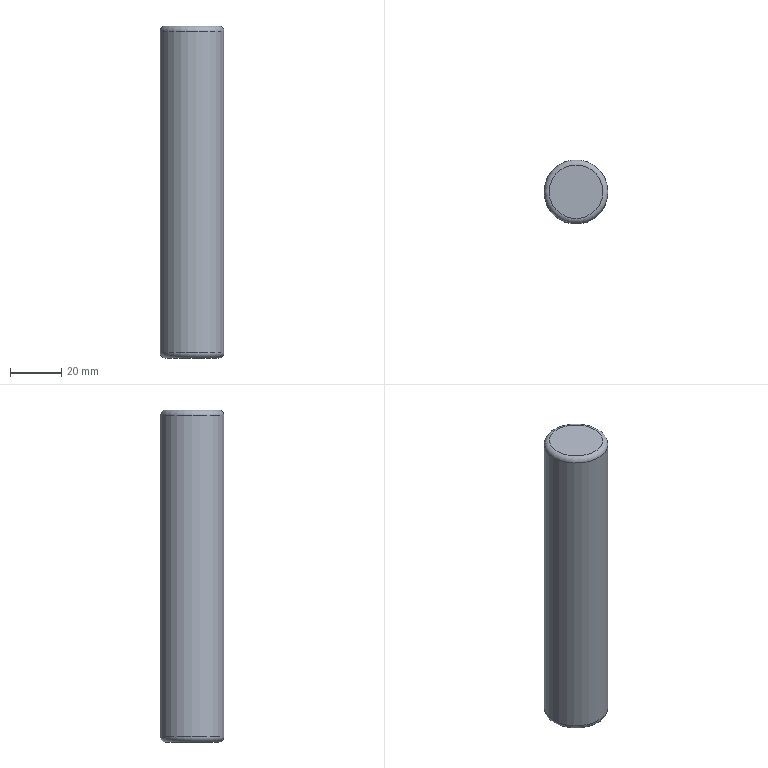Part | NX | features BLEND 1, CYLINDER 1, DATUM_CSYS 1 | 1 solid | 5 faces | box 25 x 25 x 130 mm | volume 63684 mm3 | plane 2 | torus 2 | cylinder 1 | commonest cylinder face diameters 25 x1
STEP:
#1=CARTESIAN_POINT('',(10.5,0.,130.));
#2=VERTEX_POINT('',#1);
#3=CARTESIAN_POINT('',(0.,0.,130.));
#4=DIRECTION('',(0.,0.,1.));
#5=DIRECTION('',(1.,0.,0.));
#6=AXIS2_PLACEMENT_3D('',#3,#4,#5);
#7=CIRCLE('',#6,10.5);
#8=EDGE_CURVE('',#2,#2,#7,.T.);
#9=ORIENTED_EDGE('',*,*,#8,.T.);
#10=EDGE_LOOP('',(#9));
#11=FACE_BOUND('',#10,.T.);
#12=CARTESIAN_POINT('',(0.,0.,130.));
#13=DIRECTION('',(0.,0.,1.));
#14=DIRECTION('',(1.,0.,0.));
#15=AXIS2_PLACEMENT_3D('',#12,#13,#14);
#16=PLANE('',#15);
#17=ADVANCED_FACE('',(#11),#16,.T.);
#18=CARTESIAN_POINT('',(-10.5,0.,0.));
#19=VERTEX_POINT('',#18);
#20=CARTESIAN_POINT('',(0.,0.,0.));
#21=DIRECTION('',(0.,0.,-1.));
#22=DIRECTION('',(-1.,0.,0.));
#23=AXIS2_PLACEMENT_3D('',#20,#21,#22);
#24=CIRCLE('',#23,10.5);
#25=EDGE_CURVE('',#19,#19,#24,.T.);
#26=ORIENTED_EDGE('',*,*,#25,.T.);
#27=EDGE_LOOP('',(#26));
#28=FACE_BOUND('',#27,.T.);
#29=CARTESIAN_POINT('',(0.,0.,0.));
#30=DIRECTION('',(0.,0.,-1.));
#31=DIRECTION('',(-1.,0.,0.));
#32=AXIS2_PLACEMENT_3D('',#29,#30,#31);
#33=PLANE('',#32);
#34=ADVANCED_FACE('',(#28),#33,.T.);
#35=CARTESIAN_POINT('',(-12.5,0.,2.));
#36=VERTEX_POINT('',#35);
#37=CARTESIAN_POINT('',(0.,0.,2.));
#38=DIRECTION('',(0.,0.,-1.));
#39=DIRECTION('',(-1.,0.,0.));
#40=AXIS2_PLACEMENT_3D('',#37,#38,#39);
#41=CIRCLE('',#40,12.5);
#42=EDGE_CURVE('',#36,#36,#41,.F.);
#43=ORIENTED_EDGE('',*,*,#42,.T.);
#44=EDGE_LOOP('',(#43));
#45=FACE_BOUND('',#44,.T.);
#46=CARTESIAN_POINT('',(12.5,0.,128.));
#47=VERTEX_POINT('',#46);
#48=CARTESIAN_POINT('',(0.,0.,128.));
#49=DIRECTION('',(0.,0.,1.));
#50=DIRECTION('',(1.,0.,0.));
#51=AXIS2_PLACEMENT_3D('',#48,#49,#50);
#52=CIRCLE('',#51,12.5);
#53=EDGE_CURVE('',#47,#47,#52,.F.);
#54=ORIENTED_EDGE('',*,*,#53,.T.);
#55=EDGE_LOOP('',(#54));
#56=FACE_BOUND('',#55,.T.);
#57=CARTESIAN_POINT('',(0.,0.,0.));
#58=DIRECTION('',(0.,0.,1.));
#59=DIRECTION('',(1.,0.,0.));
#60=AXIS2_PLACEMENT_3D('',#57,#58,#59);
#61=CYLINDRICAL_SURFACE('',#60,12.5);
#62=ADVANCED_FACE('',(#45,#56),#61,.T.);
#63=ORIENTED_EDGE('',*,*,#25,.F.);
#64=EDGE_LOOP('',(#63));
#65=FACE_BOUND('',#64,.T.);
#66=ORIENTED_EDGE('',*,*,#42,.F.);
#67=EDGE_LOOP('',(#66));
#68=FACE_BOUND('',#67,.T.);
#69=CARTESIAN_POINT('',(0.,0.,2.));
#70=DIRECTION('',(0.,0.,-1.));
#71=DIRECTION('',(-1.,0.,0.));
#72=AXIS2_PLACEMENT_3D('',#69,#70,#71);
#73=TOROIDAL_SURFACE('',#72,10.5,2.);
#74=ADVANCED_FACE('',(#65,#68),#73,.T.);
#75=ORIENTED_EDGE('',*,*,#8,.F.);
#76=EDGE_LOOP('',(#75));
#77=FACE_BOUND('',#76,.T.);
#78=ORIENTED_EDGE('',*,*,#53,.F.);
#79=EDGE_LOOP('',(#78));
#80=FACE_BOUND('',#79,.T.);
#81=CARTESIAN_POINT('',(0.,0.,128.));
#82=DIRECTION('',(0.,0.,1.));
#83=DIRECTION('',(1.,0.,0.));
#84=AXIS2_PLACEMENT_3D('',#81,#82,#83);
#85=TOROIDAL_SURFACE('',#84,10.5,2.);
#86=ADVANCED_FACE('',(#77,#80),#85,.T.);
#87=CLOSED_SHELL('',(#17,#34,#62,#74,#86));
#88=MANIFOLD_SOLID_BREP('',#87);
#89=(LENGTH_UNIT()NAMED_UNIT(*)SI_UNIT(.MILLI.,.METRE.));
#90=UNCERTAINTY_MEASURE_WITH_UNIT(LENGTH_MEASURE(0.00001),#89,'','');
#91=(NAMED_UNIT(*)PLANE_ANGLE_UNIT()SI_UNIT($,.RADIAN.));
#92=(NAMED_UNIT(*)SI_UNIT($,.STERADIAN.)SOLID_ANGLE_UNIT());
#93=(GEOMETRIC_REPRESENTATION_CONTEXT(3)GLOBAL_UNCERTAINTY_ASSIGNED_CONTEXT((#90))GLOBAL_UNIT_ASSIGNED_CONTEXT((#89,#91,#92))REPRESENTATION_CONTEXT('',''));
#94=ADVANCED_BREP_SHAPE_REPRESENTATION('',(#88),#93);